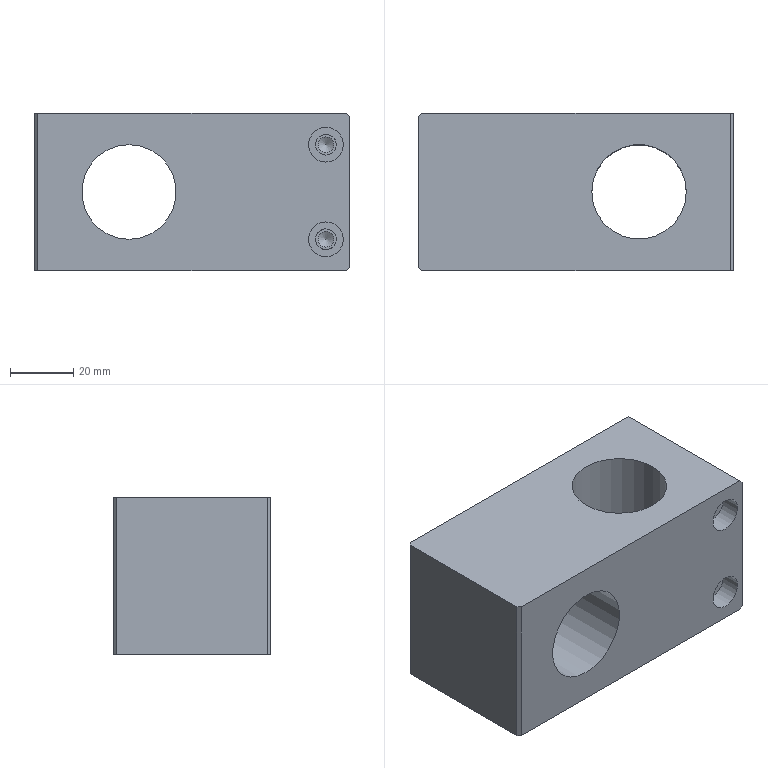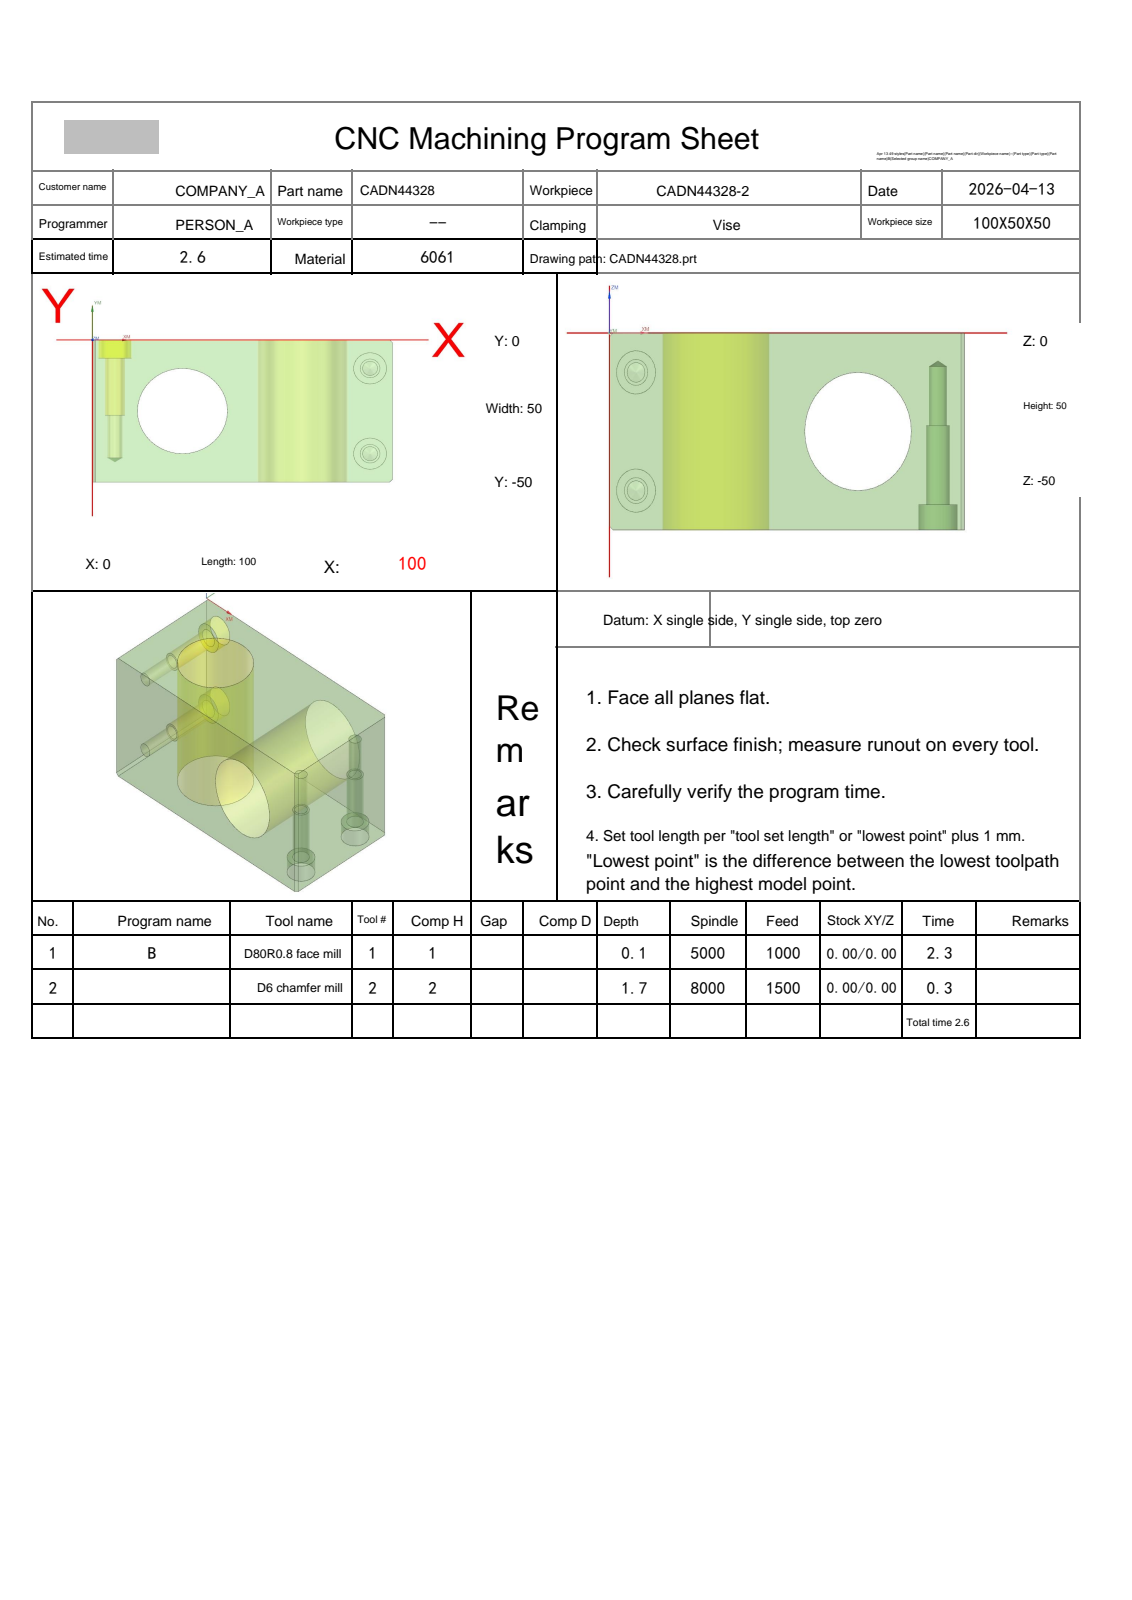NC program | NX | posted by the shop | part box 100 x 50 x 50 mm
Whole program:
%
O0001
(Machine time: 2.96 MIN)
(===Total Tool:2===)
(T1=D80R0.8 face mill D=80. R=0.8 D- H01 Z=0.    )
(T2=D6 chamfer mill D=6. R=0. D- H02 Z=-1.7  )
G80 G90 G17 G49 G40
G91 G28 Z0
M01
N1 T01 M06
(D80R0.8 face mill D=80. R=0.8 H=01 ce=0.00 di=0.10)
G00 G90 G54 X145. Y-25. M03 S5000
G43 H01 Z20.
M08
Z6.33
G01 Z4.33 F1000.
X140.
X-40.
X-45.
Z6.33
G00 Z7.8
X145.
Z5.86
G01 Z3.86
X140.
X-40.
X-45.
Z5.86
G00 Z7.33
X145.
Z5.39
G01 Z3.39
X140.
X-40.
X-45.
Z5.39
G00 Z6.86
X145.
Z4.92
G01 Z2.92
X140.
X-40.
X-45.
Z4.92
G00 Z6.39
X145.
Z4.45
G01 Z2.45
X140.
X-40.
X-45.
Z4.45
G00 Z5.92
X145.
Z3.98
G01 Z1.98
X140.
X-40.
X-45.
Z3.98
G00 Z5.45
X145.
Z3.51
G01 Z1.51
X140.
X-40.
X-45.
Z3.51
G00 Z4.98
X145.
Z3.04
G01 Z1.04
X140.
X-40.
X-45.
Z3.04
G00 Z4.51
X145.
Z2.57
G01 Z.57
X140.
X-40.
X-45.
Z2.57
G00 Z4.04
X145.
Z2.1
G01 Z.1
X140.
X-40.
X-45.
Z2.1
G00 Z20.
G00 G90 X145. Y-25. M03 S5000
Z20.
Z2.
G01 Z0.0 F1000.
X140.
X-40.
X-45.
Z2.
G00 Z20.
G91 G28 Z0.0
M05
M09
G91 G28 Z0.0
M01
N2 T02 M06
(D6 chamfer mill D=6. R=0. H=02 ce=0.00 di=0.00)
G00 G90 G54 X.508 Y.86 M03 S8000
G43 H02 Z20.
M08
Z.408
G01 Z-1.2 F1350.
X.574 Y.833
X.645 Y.83
X.667 Y.82
X.686 Y.836
X.767 Y.869 F1500.
X1. Y.9
X50.
X99.
X99.233 Y.869
X99.45 Y.779
X99.636 Y.636
X100.636 Y-.364
X100.779 Y-.55
X100.869 Y-.767
X100.9 Y-1.
Y-49.
X100.869 Y-49.233
X100.779 Y-49.45
X100.636 Y-49.636
X99.636 Y-50.636
X99.45 Y-50.779
X99.233 Y-50.869
X99. Y-50.9
X1.
X.767 Y-50.869
X.686 Y-50.836
X.667 Y-50.82
X.645 Y-50.83
X.574 Y-50.833
X.508 Y-50.86
Z.408
G00 Z10.
X29.606 Y-38.888
Z.301
G01 Z-1.2 F1350.
G03 X29.899 Y-39.077 I1.227 J1.579
G01 X29.946 Y-39.105
X30. Y-39.1
G03 X44.1 Y-25. I0.0 J14.1 F1500.
X30. Y-10.9 I-14.1 J0.0
X15.9 Y-25. I0.0 J-14.1
X30. Y-39.1 I14.1 J0.0
G01 X30.054 Y-39.105
X30.101 Y-39.077
G03 X30.394 Y-38.888 I-.935 J1.768
G01 Z.301
G00 Z20.
G00 G90 X-.708 Y-52.9 M03 S6500
Z20.
Z-.2
G01 Z-1.7 F1500.
X-.699 Y-52.832
X-.7 Y-52.763
Y2.763
X-.699 Y2.832
X-.708 Y2.9
Z-.2
G00 Z20.
M05
M09
G91 G28 Z0.0
G91 G28 Y0.0
M30
%